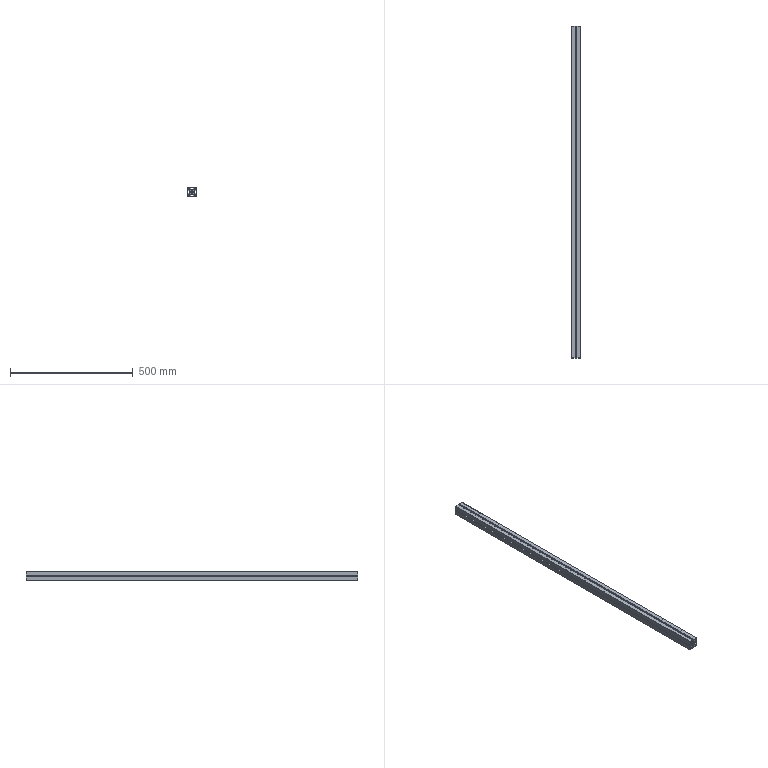Part | STEP file | 01-03 Bracket crossbar 1 | 1 solid | 68 faces | box 40 x 1350 x 40 mm | volume 1241689 mm3 | plane 54 | cylinder 14 | commonest cylinder face diameters 6 x10 2 x4